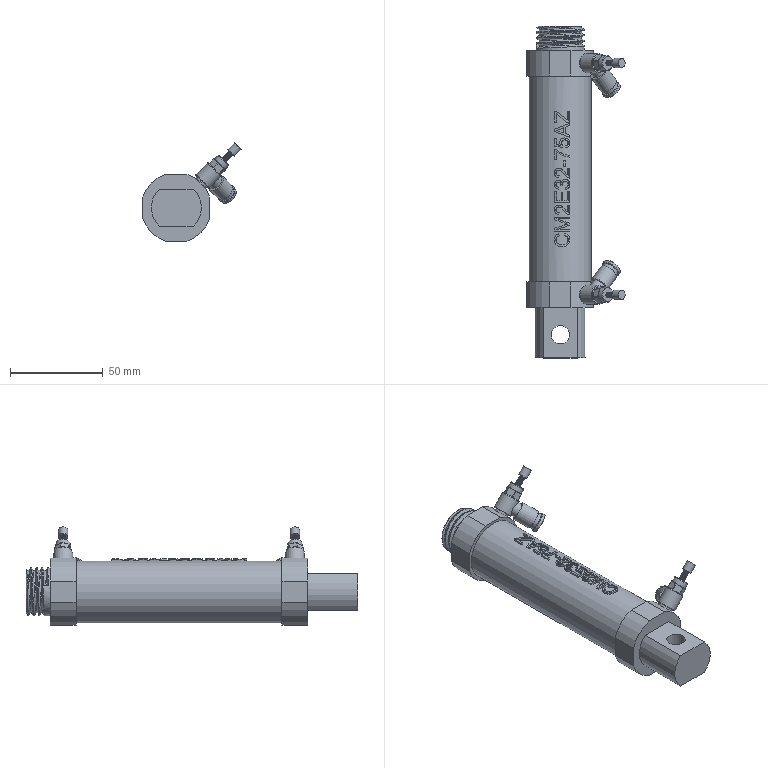Part | STEP file | Tube necking machine_id666_x_t | 1 solid | 302 faces | box 52.931 x 179 x 52.931 mm | volume 134206 mm3 | plane 190 | cylinder 52 | spline 47 | torus 12 | cone 1 | commonest cylinder face diameters 35.5 x11 37.8 x8 8 x6 10.3 x4 26 x4 2.5 x2